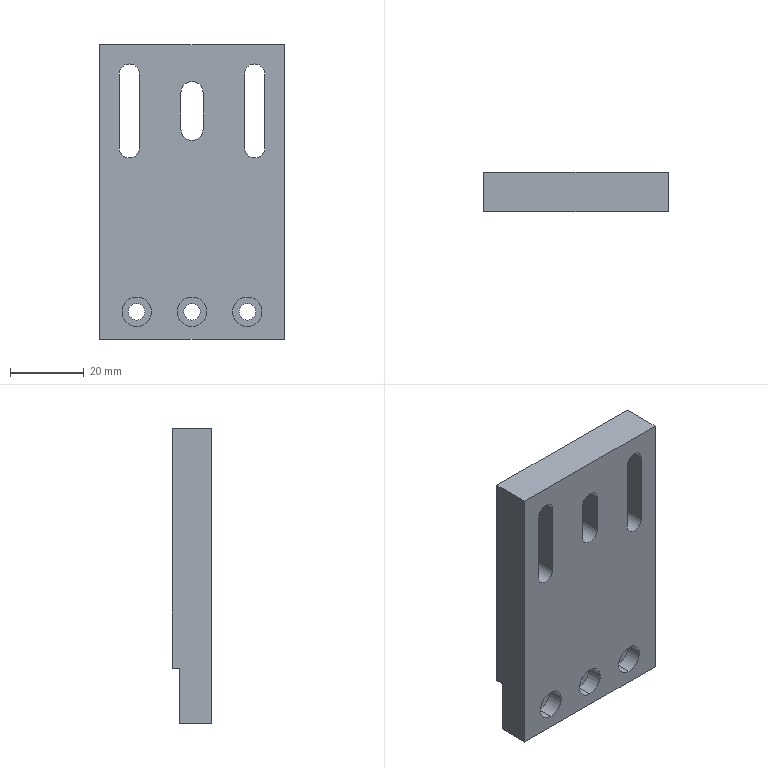Part | STEP file | 05-05 support plate | 1 solid | 50 faces | box 50 x 10.7 x 80 mm | volume 35177 mm3 | cylinder 27 | plane 23 | commonest cylinder face diameters 4.5 x6 5.5 x6 8 x6 10 x6 6 x3
STEP:
#1=CARTESIAN_POINT('',(17.,-5.35,74.75));
#2=VERTEX_POINT('',#1);
#3=CARTESIAN_POINT('',(19.75,-5.35,72.));
#4=VERTEX_POINT('',#3);
#5=CARTESIAN_POINT('',(17.,-5.35,72.));
#6=DIRECTION('',(0.,1.,0.));
#7=DIRECTION('',(0.,0.,1.));
#8=AXIS2_PLACEMENT_3D('',#5,#6,#7);
#9=CIRCLE('',#8,2.75);
#10=EDGE_CURVE('',#2,#4,#9,.T.);
#11=ORIENTED_EDGE('',*,*,#10,.F.);
#12=CARTESIAN_POINT('',(17.,0.35,74.75));
#13=VERTEX_POINT('',#12);
#14=CARTESIAN_POINT('',(17.,-10.65,74.75));
#15=DIRECTION('',(0.,1.,0.));
#16=VECTOR('',#15,1000.);
#17=LINE('',#14,#16);
#18=EDGE_CURVE('',#2,#13,#17,.T.);
#19=ORIENTED_EDGE('',*,*,#18,.T.);
#20=CARTESIAN_POINT('',(19.75,0.35,72.));
#21=VERTEX_POINT('',#20);
#22=CARTESIAN_POINT('',(17.,0.35,72.));
#23=DIRECTION('',(0.,-1.,0.));
#24=DIRECTION('',(0.,0.,-1.));
#25=AXIS2_PLACEMENT_3D('',#22,#23,#24);
#26=CIRCLE('',#25,2.75);
#27=EDGE_CURVE('',#21,#13,#26,.T.);
#28=ORIENTED_EDGE('',*,*,#27,.F.);
#29=CARTESIAN_POINT('',(19.75,-10.65,72.));
#30=DIRECTION('',(0.,1.,0.));
#31=VECTOR('',#30,1000.);
#32=LINE('',#29,#31);
#33=EDGE_CURVE('',#4,#21,#32,.T.);
#34=ORIENTED_EDGE('',*,*,#33,.F.);
#35=EDGE_LOOP('',(#11,#19,#28,#34));
#36=FACE_OUTER_BOUND('',#35,.T.);
#37=CARTESIAN_POINT('',(17.,-10.65,72.));
#38=DIRECTION('',(0.,1.,0.));
#39=DIRECTION('',(0.,0.,1.));
#40=AXIS2_PLACEMENT_3D('',#37,#38,#39);
#41=CYLINDRICAL_SURFACE('',#40,2.75);
#42=ADVANCED_FACE('',(#36),#41,.F.);
#43=CARTESIAN_POINT('',(-17.,-5.35,74.75));
#44=VERTEX_POINT('',#43);
#45=CARTESIAN_POINT('',(-14.25,-5.35,72.));
#46=VERTEX_POINT('',#45);
#47=CARTESIAN_POINT('',(-17.,-5.35,72.));
#48=DIRECTION('',(0.,1.,0.));
#49=DIRECTION('',(0.,0.,1.));
#50=AXIS2_PLACEMENT_3D('',#47,#48,#49);
#51=CIRCLE('',#50,2.75);
#52=EDGE_CURVE('',#44,#46,#51,.T.);
#53=ORIENTED_EDGE('',*,*,#52,.F.);
#54=CARTESIAN_POINT('',(-17.,0.35,74.75));
#55=VERTEX_POINT('',#54);
#56=CARTESIAN_POINT('',(-17.,-10.65,74.75));
#57=DIRECTION('',(0.,1.,0.));
#58=VECTOR('',#57,1000.);
#59=LINE('',#56,#58);
#60=EDGE_CURVE('',#44,#55,#59,.T.);
#61=ORIENTED_EDGE('',*,*,#60,.T.);
#62=CARTESIAN_POINT('',(-14.25,0.35,72.));
#63=VERTEX_POINT('',#62);
#64=CARTESIAN_POINT('',(-17.,0.35,72.));
#65=DIRECTION('',(0.,1.,0.));
#66=DIRECTION('',(0.,0.,1.));
#67=AXIS2_PLACEMENT_3D('',#64,#65,#66);
#68=CIRCLE('',#67,2.75);
#69=EDGE_CURVE('',#55,#63,#68,.T.);
#70=ORIENTED_EDGE('',*,*,#69,.T.);
#71=CARTESIAN_POINT('',(-14.25,-10.65,72.));
#72=DIRECTION('',(0.,1.,0.));
#73=VECTOR('',#72,1000.);
#74=LINE('',#71,#73);
#75=EDGE_CURVE('',#46,#63,#74,.T.);
#76=ORIENTED_EDGE('',*,*,#75,.F.);
#77=EDGE_LOOP('',(#53,#61,#70,#76));
#78=FACE_OUTER_BOUND('',#77,.T.);
#79=CARTESIAN_POINT('',(-17.,-10.65,72.));
#80=DIRECTION('',(0.,1.,0.));
#81=DIRECTION('',(0.,0.,1.));
#82=AXIS2_PLACEMENT_3D('',#79,#80,#81);
#83=CYLINDRICAL_SURFACE('',#82,2.75);
#84=ADVANCED_FACE('',(#78),#83,.F.);
#85=CARTESIAN_POINT('',(0.,-5.35,70.));
#86=VERTEX_POINT('',#85);
#87=CARTESIAN_POINT('',(3.,-5.35,67.));
#88=VERTEX_POINT('',#87);
#89=CARTESIAN_POINT('',(0.,-5.35,67.));
#90=DIRECTION('',(0.,1.,0.));
#91=DIRECTION('',(0.,0.,1.));
#92=AXIS2_PLACEMENT_3D('',#89,#90,#91);
#93=CIRCLE('',#92,3.);
#94=EDGE_CURVE('',#86,#88,#93,.T.);
#95=ORIENTED_EDGE('',*,*,#94,.F.);
#96=CARTESIAN_POINT('',(0.,5.35,70.));
#97=VERTEX_POINT('',#96);
#98=CARTESIAN_POINT('',(0.,-10.65,70.));
#99=DIRECTION('',(0.,1.,0.));
#100=VECTOR('',#99,1000.);
#101=LINE('',#98,#100);
#102=EDGE_CURVE('',#86,#97,#101,.T.);
#103=ORIENTED_EDGE('',*,*,#102,.T.);
#104=CARTESIAN_POINT('',(3.,5.35,67.));
#105=VERTEX_POINT('',#104);
#106=CARTESIAN_POINT('',(0.,5.35,67.));
#107=DIRECTION('',(0.,-1.,0.));
#108=DIRECTION('',(0.,0.,-1.));
#109=AXIS2_PLACEMENT_3D('',#106,#107,#108);
#110=CIRCLE('',#109,3.);
#111=EDGE_CURVE('',#105,#97,#110,.T.);
#112=ORIENTED_EDGE('',*,*,#111,.F.);
#113=CARTESIAN_POINT('',(3.,-10.65,67.));
#114=DIRECTION('',(0.,1.,0.));
#115=VECTOR('',#114,1000.);
#116=LINE('',#113,#115);
#117=EDGE_CURVE('',#88,#105,#116,.T.);
#118=ORIENTED_EDGE('',*,*,#117,.F.);
#119=EDGE_LOOP('',(#95,#103,#112,#118));
#120=FACE_OUTER_BOUND('',#119,.T.);
#121=CARTESIAN_POINT('',(0.,-10.65,67.));
#122=DIRECTION('',(0.,1.,0.));
#123=DIRECTION('',(0.,0.,1.));
#124=AXIS2_PLACEMENT_3D('',#121,#122,#123);
#125=CYLINDRICAL_SURFACE('',#124,3.);
#126=ADVANCED_FACE('',(#120),#125,.F.);
#127=CARTESIAN_POINT('',(17.,0.35,77.));
#128=VERTEX_POINT('',#127);
#129=CARTESIAN_POINT('',(22.,0.35,72.));
#130=VERTEX_POINT('',#129);
#131=CARTESIAN_POINT('',(17.,0.35,72.));
#132=DIRECTION('',(0.,1.,0.));
#133=DIRECTION('',(0.,0.,-1.));
#134=AXIS2_PLACEMENT_3D('',#131,#132,#133);
#135=CIRCLE('',#134,5.);
#136=EDGE_CURVE('',#128,#130,#135,.T.);
#137=ORIENTED_EDGE('',*,*,#136,.F.);
#138=CARTESIAN_POINT('',(17.,5.35,77.));
#139=VERTEX_POINT('',#138);
#140=CARTESIAN_POINT('',(17.,0.35,77.));
#141=DIRECTION('',(0.,1.,0.));
#142=VECTOR('',#141,1000.);
#143=LINE('',#140,#142);
#144=EDGE_CURVE('',#128,#139,#143,.T.);
#145=ORIENTED_EDGE('',*,*,#144,.T.);
#146=CARTESIAN_POINT('',(22.,5.35,72.));
#147=VERTEX_POINT('',#146);
#148=CARTESIAN_POINT('',(17.,5.35,72.));
#149=DIRECTION('',(0.,1.,0.));
#150=DIRECTION('',(0.,0.,-1.));
#151=AXIS2_PLACEMENT_3D('',#148,#149,#150);
#152=CIRCLE('',#151,5.);
#153=EDGE_CURVE('',#139,#147,#152,.T.);
#154=ORIENTED_EDGE('',*,*,#153,.T.);
#155=CARTESIAN_POINT('',(22.,0.35,72.));
#156=DIRECTION('',(0.,1.,0.));
#157=VECTOR('',#156,1000.);
#158=LINE('',#155,#157);
#159=EDGE_CURVE('',#130,#147,#158,.T.);
#160=ORIENTED_EDGE('',*,*,#159,.F.);
#161=EDGE_LOOP('',(#137,#145,#154,#160));
#162=FACE_OUTER_BOUND('',#161,.T.);
#163=CARTESIAN_POINT('',(17.,0.35,72.));
#164=DIRECTION('',(0.,1.,0.));
#165=DIRECTION('',(0.,0.,1.));
#166=AXIS2_PLACEMENT_3D('',#163,#164,#165);
#167=CYLINDRICAL_SURFACE('',#166,5.);
#168=ADVANCED_FACE('',(#162),#167,.F.);
#169=CARTESIAN_POINT('',(-17.,0.35,77.));
#170=VERTEX_POINT('',#169);
#171=CARTESIAN_POINT('',(-12.,0.35,72.));
#172=VERTEX_POINT('',#171);
#173=CARTESIAN_POINT('',(-17.,0.35,72.));
#174=DIRECTION('',(0.,1.,0.));
#175=DIRECTION('',(0.,0.,1.));
#176=AXIS2_PLACEMENT_3D('',#173,#174,#175);
#177=CIRCLE('',#176,5.);
#178=EDGE_CURVE('',#170,#172,#177,.T.);
#179=ORIENTED_EDGE('',*,*,#178,.F.);
#180=CARTESIAN_POINT('',(-17.,5.35,77.));
#181=VERTEX_POINT('',#180);
#182=CARTESIAN_POINT('',(-17.,0.35,77.));
#183=DIRECTION('',(0.,1.,0.));
#184=VECTOR('',#183,1000.);
#185=LINE('',#182,#184);
#186=EDGE_CURVE('',#170,#181,#185,.T.);
#187=ORIENTED_EDGE('',*,*,#186,.T.);
#188=CARTESIAN_POINT('',(-12.,5.35,72.));
#189=VERTEX_POINT('',#188);
#190=CARTESIAN_POINT('',(-17.,5.35,72.));
#191=DIRECTION('',(0.,1.,0.));
#192=DIRECTION('',(0.,0.,1.));
#193=AXIS2_PLACEMENT_3D('',#190,#191,#192);
#194=CIRCLE('',#193,5.);
#195=EDGE_CURVE('',#181,#189,#194,.T.);
#196=ORIENTED_EDGE('',*,*,#195,.T.);
#197=CARTESIAN_POINT('',(-12.,0.35,72.));
#198=DIRECTION('',(0.,1.,0.));
#199=VECTOR('',#198,1000.);
#200=LINE('',#197,#199);
#201=EDGE_CURVE('',#172,#189,#200,.T.);
#202=ORIENTED_EDGE('',*,*,#201,.F.);
#203=EDGE_LOOP('',(#179,#187,#196,#202));
#204=FACE_OUTER_BOUND('',#203,.T.);
#205=CARTESIAN_POINT('',(-17.,0.35,72.));
#206=DIRECTION('',(0.,1.,0.));
#207=DIRECTION('',(0.,0.,1.));
#208=AXIS2_PLACEMENT_3D('',#205,#206,#207);
#209=CYLINDRICAL_SURFACE('',#208,5.);
#210=ADVANCED_FACE('',(#204),#209,.F.);
#211=CARTESIAN_POINT('',(15.,-0.95,11.5));
#212=VERTEX_POINT('',#211);
#213=CARTESIAN_POINT('',(15.,-0.95,3.5));
#214=VERTEX_POINT('',#213);
#215=CARTESIAN_POINT('',(15.,-0.95,7.5));
#216=DIRECTION('',(0.,-1.,0.));
#217=DIRECTION('',(0.,0.,-1.));
#218=AXIS2_PLACEMENT_3D('',#215,#216,#217);
#219=CIRCLE('',#218,4.);
#220=EDGE_CURVE('',#212,#214,#219,.T.);
#221=ORIENTED_EDGE('',*,*,#220,.F.);
#222=CARTESIAN_POINT('',(15.,-5.35,11.5));
#223=VERTEX_POINT('',#222);
#224=CARTESIAN_POINT('',(15.,-5.35,11.5));
#225=DIRECTION('',(0.,-1.,0.));
#226=VECTOR('',#225,1000.);
#227=LINE('',#224,#226);
#228=EDGE_CURVE('',#212,#223,#227,.T.);
#229=ORIENTED_EDGE('',*,*,#228,.T.);
#230=CARTESIAN_POINT('',(15.,-5.35,3.5));
#231=VERTEX_POINT('',#230);
#232=CARTESIAN_POINT('',(15.,-5.35,7.5));
#233=DIRECTION('',(0.,-1.,0.));
#234=DIRECTION('',(0.,0.,-1.));
#235=AXIS2_PLACEMENT_3D('',#232,#233,#234);
#236=CIRCLE('',#235,4.);
#237=EDGE_CURVE('',#223,#231,#236,.T.);
#238=ORIENTED_EDGE('',*,*,#237,.T.);
#239=CARTESIAN_POINT('',(15.,-5.35,3.5));
#240=DIRECTION('',(0.,-1.,0.));
#241=VECTOR('',#240,1000.);
#242=LINE('',#239,#241);
#243=EDGE_CURVE('',#214,#231,#242,.T.);
#244=ORIENTED_EDGE('',*,*,#243,.F.);
#245=EDGE_LOOP('',(#221,#229,#238,#244));
#246=FACE_OUTER_BOUND('',#245,.T.);
#247=CARTESIAN_POINT('',(15.,-5.35,7.5));
#248=DIRECTION('',(0.,-1.,0.));
#249=DIRECTION('',(0.,0.,-1.));
#250=AXIS2_PLACEMENT_3D('',#247,#248,#249);
#251=CYLINDRICAL_SURFACE('',#250,4.);
#252=ADVANCED_FACE('',(#246),#251,.F.);
#253=CARTESIAN_POINT('',(15.,3.35,9.75));
#254=VERTEX_POINT('',#253);
#255=CARTESIAN_POINT('',(15.,3.35,5.25));
#256=VERTEX_POINT('',#255);
#257=CARTESIAN_POINT('',(15.,3.35,7.5));
#258=DIRECTION('',(0.,-1.,0.));
#259=DIRECTION('',(1.,0.,0.));
#260=AXIS2_PLACEMENT_3D('',#257,#258,#259);
#261=CIRCLE('',#260,2.25);
#262=EDGE_CURVE('',#254,#256,#261,.T.);
#263=ORIENTED_EDGE('',*,*,#262,.F.);
#264=CARTESIAN_POINT('',(15.,-0.95,9.75));
#265=VERTEX_POINT('',#264);
#266=CARTESIAN_POINT('',(15.,-5.35,9.75));
#267=DIRECTION('',(0.,-1.,0.));
#268=VECTOR('',#267,1000.);
#269=LINE('',#266,#268);
#270=EDGE_CURVE('',#254,#265,#269,.T.);
#271=ORIENTED_EDGE('',*,*,#270,.T.);
#272=CARTESIAN_POINT('',(15.,-0.95,5.25));
#273=VERTEX_POINT('',#272);
#274=CARTESIAN_POINT('',(15.,-0.95,7.5));
#275=DIRECTION('',(0.,-1.,0.));
#276=DIRECTION('',(0.,0.,-1.));
#277=AXIS2_PLACEMENT_3D('',#274,#275,#276);
#278=CIRCLE('',#277,2.25);
#279=EDGE_CURVE('',#265,#273,#278,.T.);
#280=ORIENTED_EDGE('',*,*,#279,.T.);
#281=CARTESIAN_POINT('',(15.,-5.35,5.25));
#282=DIRECTION('',(0.,-1.,0.));
#283=VECTOR('',#282,1000.);
#284=LINE('',#281,#283);
#285=EDGE_CURVE('',#256,#273,#284,.T.);
#286=ORIENTED_EDGE('',*,*,#285,.F.);
#287=EDGE_LOOP('',(#263,#271,#280,#286));
#288=FACE_OUTER_BOUND('',#287,.T.);
#289=CARTESIAN_POINT('',(15.,-5.35,7.5));
#290=DIRECTION('',(0.,-1.,0.));
#291=DIRECTION('',(0.,0.,-1.));
#292=AXIS2_PLACEMENT_3D('',#289,#290,#291);
#293=CYLINDRICAL_SURFACE('',#292,2.25);
#294=ADVANCED_FACE('',(#288),#293,.F.);
#295=CARTESIAN_POINT('',(0.,-0.95,11.5));
#296=VERTEX_POINT('',#295);
#297=CARTESIAN_POINT('',(0.,-0.95,3.5));
#298=VERTEX_POINT('',#297);
#299=CARTESIAN_POINT('',(0.,-0.95,7.5));
#300=DIRECTION('',(0.,-1.,0.));
#301=DIRECTION('',(0.,0.,-1.));
#302=AXIS2_PLACEMENT_3D('',#299,#300,#301);
#303=CIRCLE('',#302,4.);
#304=EDGE_CURVE('',#296,#298,#303,.T.);
#305=ORIENTED_EDGE('',*,*,#304,.F.);
#306=CARTESIAN_POINT('',(0.,-5.35,11.5));
#307=VERTEX_POINT('',#306);
#308=CARTESIAN_POINT('',(0.,-5.35,11.5));
#309=DIRECTION('',(0.,-1.,0.));
#310=VECTOR('',#309,1000.);
#311=LINE('',#308,#310);
#312=EDGE_CURVE('',#296,#307,#311,.T.);
#313=ORIENTED_EDGE('',*,*,#312,.T.);
#314=CARTESIAN_POINT('',(0.,-5.35,3.5));
#315=VERTEX_POINT('',#314);
#316=CARTESIAN_POINT('',(0.,-5.35,7.5));
#317=DIRECTION('',(0.,-1.,0.));
#318=DIRECTION('',(0.,0.,-1.));
#319=AXIS2_PLACEMENT_3D('',#316,#317,#318);
#320=CIRCLE('',#319,4.);
#321=EDGE_CURVE('',#307,#315,#320,.T.);
#322=ORIENTED_EDGE('',*,*,#321,.T.);
#323=CARTESIAN_POINT('',(0.,-5.35,3.5));
#324=DIRECTION('',(0.,-1.,0.));
#325=VECTOR('',#324,1000.);
#326=LINE('',#323,#325);
#327=EDGE_CURVE('',#298,#315,#326,.T.);
#328=ORIENTED_EDGE('',*,*,#327,.F.);
#329=EDGE_LOOP('',(#305,#313,#322,#328));
#330=FACE_OUTER_BOUND('',#329,.T.);
#331=CARTESIAN_POINT('',(0.,-5.35,7.5));
#332=DIRECTION('',(0.,-1.,0.));
#333=DIRECTION('',(0.,0.,-1.));
#334=AXIS2_PLACEMENT_3D('',#331,#332,#333);
#335=CYLINDRICAL_SURFACE('',#334,4.);
#336=ADVANCED_FACE('',(#330),#335,.F.);
#337=CARTESIAN_POINT('',(0.,3.35,9.75));
#338=VERTEX_POINT('',#337);
#339=CARTESIAN_POINT('',(0.,3.35,5.25));
#340=VERTEX_POINT('',#339);
#341=CARTESIAN_POINT('',(0.,3.35,7.5));
#342=DIRECTION('',(0.,-1.,0.));
#343=DIRECTION('',(1.,0.,0.));
#344=AXIS2_PLACEMENT_3D('',#341,#342,#343);
#345=CIRCLE('',#344,2.25);
#346=EDGE_CURVE('',#338,#340,#345,.T.);
#347=ORIENTED_EDGE('',*,*,#346,.F.);
#348=CARTESIAN_POINT('',(0.,-0.95,9.75));
#349=VERTEX_POINT('',#348);
#350=CARTESIAN_POINT('',(0.,-5.35,9.75));
#351=DIRECTION('',(0.,-1.,0.));
#352=VECTOR('',#351,1000.);
#353=LINE('',#350,#352);
#354=EDGE_CURVE('',#338,#349,#353,.T.);
#355=ORIENTED_EDGE('',*,*,#354,.T.);
#356=CARTESIAN_POINT('',(0.,-0.95,5.25));
#357=VERTEX_POINT('',#356);
#358=CARTESIAN_POINT('',(0.,-0.95,7.5));
#359=DIRECTION('',(0.,-1.,0.));
#360=DIRECTION('',(0.,0.,-1.));
#361=AXIS2_PLACEMENT_3D('',#358,#359,#360);
#362=CIRCLE('',#361,2.25);
#363=EDGE_CURVE('',#349,#357,#362,.T.);
#364=ORIENTED_EDGE('',*,*,#363,.T.);
#365=CARTESIAN_POINT('',(0.,-5.35,5.25));
#366=DIRECTION('',(0.,-1.,0.));
#367=VECTOR('',#366,1000.);
#368=LINE('',#365,#367);
#369=EDGE_CURVE('',#340,#357,#368,.T.);
#370=ORIENTED_EDGE('',*,*,#369,.F.);
#371=EDGE_LOOP('',(#347,#355,#364,#370));
#372=FACE_OUTER_BOUND('',#371,.T.);
#373=CARTESIAN_POINT('',(0.,-5.35,7.5));
#374=DIRECTION('',(0.,-1.,0.));
#375=DIRECTION('',(0.,0.,-1.));
#376=AXIS2_PLACEMENT_3D('',#373,#374,#375);
#377=CYLINDRICAL_SURFACE('',#376,2.25);
#378=ADVANCED_FACE('',(#372),#377,.F.);
#379=CARTESIAN_POINT('',(-15.,-0.95,11.5));
#380=VERTEX_POINT('',#379);
#381=CARTESIAN_POINT('',(-15.,-0.95,3.5));
#382=VERTEX_POINT('',#381);
#383=CARTESIAN_POINT('',(-15.,-0.95,7.5));
#384=DIRECTION('',(0.,-1.,0.));
#385=DIRECTION('',(0.,0.,-1.));
#386=AXIS2_PLACEMENT_3D('',#383,#384,#385);
#387=CIRCLE('',#386,4.);
#388=EDGE_CURVE('',#380,#382,#387,.T.);
#389=ORIENTED_EDGE('',*,*,#388,.F.);
#390=CARTESIAN_POINT('',(-15.,-5.35,11.5));
#391=VERTEX_POINT('',#390);
#392=CARTESIAN_POINT('',(-15.,-5.35,11.5));
#393=DIRECTION('',(0.,-1.,0.));
#394=VECTOR('',#393,1000.);
#395=LINE('',#392,#394);
#396=EDGE_CURVE('',#380,#391,#395,.T.);
#397=ORIENTED_EDGE('',*,*,#396,.T.);
#398=CARTESIAN_POINT('',(-15.,-5.35,3.5));
#399=VERTEX_POINT('',#398);
#400=CARTESIAN_POINT('',(-15.,-5.35,7.5));
#401=DIRECTION('',(0.,-1.,0.));
#402=DIRECTION('',(0.,0.,-1.));
#403=AXIS2_PLACEMENT_3D('',#400,#401,#402);
#404=CIRCLE('',#403,4.);
#405=EDGE_CURVE('',#391,#399,#404,.T.);
#406=ORIENTED_EDGE('',*,*,#405,.T.);
#407=CARTESIAN_POINT('',(-15.,-5.35,3.5));
#408=DIRECTION('',(0.,-1.,0.));
#409=VECTOR('',#408,1000.);
#410=LINE('',#407,#409);
#411=EDGE_CURVE('',#382,#399,#410,.T.);
#412=ORIENTED_EDGE('',*,*,#411,.F.);
#413=EDGE_LOOP('',(#389,#397,#406,#412));
#414=FACE_OUTER_BOUND('',#413,.T.);
#415=CARTESIAN_POINT('',(-15.,-5.35,7.5));
#416=DIRECTION('',(0.,-1.,0.));
#417=DIRECTION('',(0.,0.,-1.));
#418=AXIS2_PLACEMENT_3D('',#415,#416,#417);
#419=CYLINDRICAL_SURFACE('',#418,4.);
#420=ADVANCED_FACE('',(#414),#419,.F.);
#421=CARTESIAN_POINT('',(-15.,3.35,9.75));
#422=VERTEX_POINT('',#421);
#423=CARTESIAN_POINT('',(-15.,3.35,5.25));
#424=VERTEX_POINT('',#423);
#425=CARTESIAN_POINT('',(-15.,3.35,7.5));
#426=DIRECTION('',(0.,-1.,0.));
#427=DIRECTION('',(1.,0.,0.));
#428=AXIS2_PLACEMENT_3D('',#425,#426,#427);
#429=CIRCLE('',#428,2.25);
#430=EDGE_CURVE('',#422,#424,#429,.T.);
#431=ORIENTED_EDGE('',*,*,#430,.F.);
#432=CARTESIAN_POINT('',(-15.,-0.95,9.75));
#433=VERTEX_POINT('',#432);
#434=CARTESIAN_POINT('',(-15.,-5.35,9.75));
#435=DIRECTION('',(0.,-1.,0.));
#436=VECTOR('',#435,1000.);
#437=LINE('',#434,#436);
#438=EDGE_CURVE('',#422,#433,#437,.T.);
#439=ORIENTED_EDGE('',*,*,#438,.T.);
#440=CARTESIAN_POINT('',(-15.,-0.95,5.25));
#441=VERTEX_POINT('',#440);
#442=CARTESIAN_POINT('',(-15.,-0.95,7.5));
#443=DIRECTION('',(0.,-1.,0.));
#444=DIRECTION('',(0.,0.,-1.));
#445=AXIS2_PLACEMENT_3D('',#442,#443,#444);
#446=CIRCLE('',#445,2.25);
#447=EDGE_CURVE('',#433,#441,#446,.T.);
#448=ORIENTED_EDGE('',*,*,#447,.T.);
#449=CARTESIAN_POINT('',(-15.,-5.35,5.25));
#450=DIRECTION('',(0.,-1.,0.));
#451=VECTOR('',#450,1000.);
#452=LINE('',#449,#451);
#453=EDGE_CURVE('',#424,#441,#452,.T.);
#454=ORIENTED_EDGE('',*,*,#453,.F.);
#455=EDGE_LOOP('',(#431,#439,#448,#454));
#456=FACE_OUTER_BOUND('',#455,.T.);
#457=CARTESIAN_POINT('',(-15.,-5.35,7.5));
#458=DIRECTION('',(0.,-1.,0.));
#459=DIRECTION('',(0.,0.,-1.));
#460=AXIS2_PLACEMENT_3D('',#457,#458,#459);
#461=CYLINDRICAL_SURFACE('',#460,2.25);
#462=ADVANCED_FACE('',(#456),#461,.F.);
#463=CARTESIAN_POINT('',(25.,-5.35,0.));
#464=VERTEX_POINT('',#463);
#465=CARTESIAN_POINT('',(25.,3.35,0.));
#466=VERTEX_POINT('',#465);
#467=CARTESIAN_POINT('',(25.,5.35,0.));
#468=DIRECTION('',(0.,1.,0.));
#469=VECTOR('',#468,1000.);
#470=LINE('',#467,#469);
#471=EDGE_CURVE('',#464,#466,#470,.T.);
#472=ORIENTED_EDGE('',*,*,#471,.T.);
#473=CARTESIAN_POINT('',(25.,3.35,15.));
#474=VERTEX_POINT('',#473);
#475=CARTESIAN_POINT('',(25.,3.35,0.));
#476=DIRECTION('',(0.,0.,-1.));
#477=VECTOR('',#476,1000.);
#478=LINE('',#475,#477);
#479=EDGE_CURVE('',#474,#466,#478,.T.);
#480=ORIENTED_EDGE('',*,*,#479,.F.);
#481=CARTESIAN_POINT('',(25.,5.35,15.));
#482=VERTEX_POINT('',#481);
#483=CARTESIAN_POINT('',(25.,5.35,15.));
#484=DIRECTION('',(0.,-1.,0.));
#485=VECTOR('',#484,1000.);
#486=LINE('',#483,#485);
#487=EDGE_CURVE('',#482,#474,#486,.T.);
#488=ORIENTED_EDGE('',*,*,#487,.F.);
#489=CARTESIAN_POINT('',(25.,5.35,80.));
#490=VERTEX_POINT('',#489);
#491=CARTESIAN_POINT('',(25.,5.35,80.));
#492=DIRECTION('',(0.,0.,-1.));
#493=VECTOR('',#492,1000.);
#494=LINE('',#491,#493);
#495=EDGE_CURVE('',#490,#482,#494,.T.);
#496=ORIENTED_EDGE('',*,*,#495,.F.);
#497=CARTESIAN_POINT('',(25.,-5.35,80.));
#498=VERTEX_POINT('',#497);
#499=CARTESIAN_POINT('',(25.,5.35,80.));
#500=DIRECTION('',(0.,1.,0.));
#501=VECTOR('',#500,1000.);
#502=LINE('',#499,#501);
#503=EDGE_CURVE('',#498,#490,#502,.T.);
#504=ORIENTED_EDGE('',*,*,#503,.F.);
#505=CARTESIAN_POINT('',(25.,-5.35,80.));
#506=DIRECTION('',(0.,0.,-1.));
#507=VECTOR('',#506,1000.);
#508=LINE('',#505,#507);
#509=EDGE_CURVE('',#498,#464,#508,.T.);
#510=ORIENTED_EDGE('',*,*,#509,.T.);
#511=EDGE_LOOP('',(#472,#480,#488,#496,#504,#510));
#512=FACE_OUTER_BOUND('',#511,.T.);
#513=CARTESIAN_POINT('',(25.,5.35,80.));
#514=DIRECTION('',(-1.,0.,0.));
#515=DIRECTION('',(0.,-1.,0.));
#516=AXIS2_PLACEMENT_3D('',#513,#514,#515);
#517=PLANE('',#516);
#518=ADVANCED_FACE('',(#512),#517,.F.);
#519=CARTESIAN_POINT('',(-3.,5.35,67.));
#520=VERTEX_POINT('',#519);
#521=CARTESIAN_POINT('',(-3.,5.35,57.));
#522=VERTEX_POINT('',#521);
#523=CARTESIAN_POINT('',(-3.,5.35,80.));
#524=DIRECTION('',(0.,0.,-1.));
#525=VECTOR('',#524,1000.);
#526=LINE('',#523,#525);
#527=EDGE_CURVE('',#520,#522,#526,.T.);
#528=ORIENTED_EDGE('',*,*,#527,.T.);
#529=CARTESIAN_POINT('',(3.,5.35,57.));
#530=VERTEX_POINT('',#529);
#531=CARTESIAN_POINT('',(0.,5.35,57.));
#532=DIRECTION('',(0.,-1.,0.));
#533=DIRECTION('',(0.,0.,-1.));
#534=AXIS2_PLACEMENT_3D('',#531,#532,#533);
#535=CIRCLE('',#534,3.);
#536=EDGE_CURVE('',#522,#530,#535,.T.);
#537=ORIENTED_EDGE('',*,*,#536,.T.);
#538=CARTESIAN_POINT('',(3.,5.35,80.));
#539=DIRECTION('',(0.,0.,1.));
#540=VECTOR('',#539,1000.);
#541=LINE('',#538,#540);
#542=EDGE_CURVE('',#530,#105,#541,.T.);
#543=ORIENTED_EDGE('',*,*,#542,.T.);
#544=ORIENTED_EDGE('',*,*,#111,.T.);
#545=CARTESIAN_POINT('',(0.,5.35,67.));
#546=DIRECTION('',(0.,-1.,0.));
#547=DIRECTION('',(0.,0.,-1.));
#548=AXIS2_PLACEMENT_3D('',#545,#546,#547);
#549=CIRCLE('',#548,3.);
#550=EDGE_CURVE('',#97,#520,#549,.T.);
#551=ORIENTED_EDGE('',*,*,#550,.T.);
#552=EDGE_LOOP('',(#528,#537,#543,#544,#551));
#553=FACE_BOUND('',#552,.T.);
#554=CARTESIAN_POINT('',(12.,5.35,52.));
#555=VERTEX_POINT('',#554);
#556=CARTESIAN_POINT('',(12.,5.35,72.));
#557=VERTEX_POINT('',#556);
#558=CARTESIAN_POINT('',(12.,5.35,52.));
#559=DIRECTION('',(0.,0.,1.));
#560=VECTOR('',#559,1000.);
#561=LINE('',#558,#560);
#562=EDGE_CURVE('',#555,#557,#561,.T.);
#563=ORIENTED_EDGE('',*,*,#562,.F.);
#564=CARTESIAN_POINT('',(22.,5.35,52.));
#565=VERTEX_POINT('',#564);
#566=CARTESIAN_POINT('',(17.,5.35,52.));
#567=DIRECTION('',(0.,1.,0.));
#568=DIRECTION('',(0.,0.,-1.));
#569=AXIS2_PLACEMENT_3D('',#566,#567,#568);
#570=CIRCLE('',#569,5.);
#571=EDGE_CURVE('',#565,#555,#570,.T.);
#572=ORIENTED_EDGE('',*,*,#571,.F.);
#573=CARTESIAN_POINT('',(22.,5.35,52.));
#574=DIRECTION('',(0.,0.,-1.));
#575=VECTOR('',#574,1000.);
#576=LINE('',#573,#575);
#577=EDGE_CURVE('',#147,#565,#576,.T.);
#578=ORIENTED_EDGE('',*,*,#577,.F.);
#579=ORIENTED_EDGE('',*,*,#153,.F.);
#580=CARTESIAN_POINT('',(17.,5.35,72.));
#581=DIRECTION('',(0.,1.,0.));
#582=DIRECTION('',(0.,0.,-1.));
#583=AXIS2_PLACEMENT_3D('',#580,#581,#582);
#584=CIRCLE('',#583,5.);
#585=EDGE_CURVE('',#557,#139,#584,.T.);
#586=ORIENTED_EDGE('',*,*,#585,.F.);
#587=EDGE_LOOP('',(#563,#572,#578,#579,#586));
#588=FACE_BOUND('',#587,.T.);
#589=CARTESIAN_POINT('',(-22.,5.35,52.));
#590=VERTEX_POINT('',#589);
#591=CARTESIAN_POINT('',(-22.,5.35,72.));
#592=VERTEX_POINT('',#591);
#593=CARTESIAN_POINT('',(-22.,5.35,52.));
#594=DIRECTION('',(0.,0.,1.));
#595=VECTOR('',#594,1000.);
#596=LINE('',#593,#595);
#597=EDGE_CURVE('',#590,#592,#596,.T.);
#598=ORIENTED_EDGE('',*,*,#597,.F.);
#599=CARTESIAN_POINT('',(-12.,5.35,52.));
#600=VERTEX_POINT('',#599);
#601=CARTESIAN_POINT('',(-17.,5.35,52.));
#602=DIRECTION('',(0.,1.,0.));
#603=DIRECTION('',(0.,0.,1.));
#604=AXIS2_PLACEMENT_3D('',#601,#602,#603);
#605=CIRCLE('',#604,5.);
#606=EDGE_CURVE('',#600,#590,#605,.T.);
#607=ORIENTED_EDGE('',*,*,#606,.F.);
#608=CARTESIAN_POINT('',(-12.,5.35,52.));
#609=DIRECTION('',(0.,0.,-1.));
#610=VECTOR('',#609,1000.);
#611=LINE('',#608,#610);
#612=EDGE_CURVE('',#189,#600,#611,.T.);
#613=ORIENTED_EDGE('',*,*,#612,.F.);
#614=ORIENTED_EDGE('',*,*,#195,.F.);
#615=CARTESIAN_POINT('',(-17.,5.35,72.));
#616=DIRECTION('',(0.,1.,0.));
#617=DIRECTION('',(0.,0.,1.));
#618=AXIS2_PLACEMENT_3D('',#615,#616,#617);
#619=CIRCLE('',#618,5.);
#620=EDGE_CURVE('',#592,#181,#619,.T.);
#621=ORIENTED_EDGE('',*,*,#620,.F.);
#622=EDGE_LOOP('',(#598,#607,#613,#614,#621));
#623=FACE_BOUND('',#622,.T.);
#624=ORIENTED_EDGE('',*,*,#495,.T.);
#625=CARTESIAN_POINT('',(-25.,5.35,15.));
#626=VERTEX_POINT('',#625);
#627=CARTESIAN_POINT('',(-35.,5.35,15.));
#628=DIRECTION('',(1.,0.,0.));
#629=VECTOR('',#628,1000.);
#630=LINE('',#627,#629);
#631=EDGE_CURVE('',#626,#482,#630,.T.);
#632=ORIENTED_EDGE('',*,*,#631,.F.);
#633=CARTESIAN_POINT('',(-25.,5.35,80.));
#634=VERTEX_POINT('',#633);
#635=CARTESIAN_POINT('',(-25.,5.35,80.));
#636=DIRECTION('',(0.,0.,-1.));
#637=VECTOR('',#636,1000.);
#638=LINE('',#635,#637);
#639=EDGE_CURVE('',#634,#626,#638,.T.);
#640=ORIENTED_EDGE('',*,*,#639,.F.);
#641=CARTESIAN_POINT('',(-25.,5.35,80.));
#642=DIRECTION('',(-1.,0.,0.));
#643=VECTOR('',#642,1000.);
#644=LINE('',#641,#643);
#645=EDGE_CURVE('',#490,#634,#644,.T.);
#646=ORIENTED_EDGE('',*,*,#645,.F.);
#647=EDGE_LOOP('',(#624,#632,#640,#646));
#648=FACE_OUTER_BOUND('',#647,.T.);
#649=CARTESIAN_POINT('',(-25.,5.35,80.));
#650=DIRECTION('',(0.,-1.,0.));
#651=DIRECTION('',(0.,0.,-1.));
#652=AXIS2_PLACEMENT_3D('',#649,#650,#651);
#653=PLANE('',#652);
#654=ADVANCED_FACE('',(#553,#588,#623,#648),#653,.F.);
#655=CARTESIAN_POINT('',(-25.,3.35,15.));
#656=VERTEX_POINT('',#655);
#657=CARTESIAN_POINT('',(-25.,5.35,15.));
#658=DIRECTION('',(0.,-1.,0.));
#659=VECTOR('',#658,1000.);
#660=LINE('',#657,#659);
#661=EDGE_CURVE('',#626,#656,#660,.T.);
#662=ORIENTED_EDGE('',*,*,#661,.T.);
#663=CARTESIAN_POINT('',(-25.,3.35,0.));
#664=VERTEX_POINT('',#663);
#665=CARTESIAN_POINT('',(-25.,3.35,80.));
#666=DIRECTION('',(0.,0.,-1.));
#667=VECTOR('',#666,1000.);
#668=LINE('',#665,#667);
#669=EDGE_CURVE('',#656,#664,#668,.T.);
#670=ORIENTED_EDGE('',*,*,#669,.T.);
#671=CARTESIAN_POINT('',(-25.,-5.35,0.));
#672=VERTEX_POINT('',#671);
#673=CARTESIAN_POINT('',(-25.,5.35,0.));
#674=DIRECTION('',(0.,-1.,0.));
#675=VECTOR('',#674,1000.);
#676=LINE('',#673,#675);
#677=EDGE_CURVE('',#664,#672,#676,.T.);
#678=ORIENTED_EDGE('',*,*,#677,.T.);
#679=CARTESIAN_POINT('',(-25.,-5.35,80.));
#680=VERTEX_POINT('',#679);
#681=CARTESIAN_POINT('',(-25.,-5.35,80.));
#682=DIRECTION('',(0.,0.,-1.));
#683=VECTOR('',#682,1000.);
#684=LINE('',#681,#683);
#685=EDGE_CURVE('',#680,#672,#684,.T.);
#686=ORIENTED_EDGE('',*,*,#685,.F.);
#687=CARTESIAN_POINT('',(-25.,5.35,80.));
#688=DIRECTION('',(0.,-1.,0.));
#689=VECTOR('',#688,1000.);
#690=LINE('',#687,#689);
#691=EDGE_CURVE('',#634,#680,#690,.T.);
#692=ORIENTED_EDGE('',*,*,#691,.F.);
#693=ORIENTED_EDGE('',*,*,#639,.T.);
#694=EDGE_LOOP('',(#662,#670,#678,#686,#692,#693));
#695=FACE_OUTER_BOUND('',#694,.T.);
#696=CARTESIAN_POINT('',(-25.,5.35,80.));
#697=DIRECTION('',(1.,0.,0.));
#698=DIRECTION('',(0.,0.,-1.));
#699=AXIS2_PLACEMENT_3D('',#696,#697,#698);
#700=PLANE('',#699);
#701=ADVANCED_FACE('',(#695),#700,.F.);
#702=CARTESIAN_POINT('',(19.75,-5.35,52.));
#703=VERTEX_POINT('',#702);
#704=CARTESIAN_POINT('',(19.75,-5.35,80.));
#705=DIRECTION('',(0.,0.,-1.));
#706=VECTOR('',#705,1000.);
#707=LINE('',#704,#706);
#708=EDGE_CURVE('',#4,#703,#707,.T.);
#709=ORIENTED_EDGE('',*,*,#708,.T.);
#710=CARTESIAN_POINT('',(14.25,-5.35,52.));
#711=VERTEX_POINT('',#710);
#712=CARTESIAN_POINT('',(17.,-5.35,52.));
#713=DIRECTION('',(0.,1.,0.));
#714=DIRECTION('',(0.,0.,1.));
#715=AXIS2_PLACEMENT_3D('',#712,#713,#714);
#716=CIRCLE('',#715,2.75);
#717=EDGE_CURVE('',#703,#711,#716,.T.);
#718=ORIENTED_EDGE('',*,*,#717,.T.);
#719=CARTESIAN_POINT('',(14.25,-5.35,72.));
#720=VERTEX_POINT('',#719);
#721=CARTESIAN_POINT('',(14.25,-5.35,80.));
#722=DIRECTION('',(0.,0.,1.));
#723=VECTOR('',#722,1000.);
#724=LINE('',#721,#723);
#725=EDGE_CURVE('',#711,#720,#724,.T.);
#726=ORIENTED_EDGE('',*,*,#725,.T.);
#727=CARTESIAN_POINT('',(17.,-5.35,72.));
#728=DIRECTION('',(0.,1.,0.));
#729=DIRECTION('',(0.,0.,1.));
#730=AXIS2_PLACEMENT_3D('',#727,#728,#729);
#731=CIRCLE('',#730,2.75);
#732=EDGE_CURVE('',#720,#2,#731,.T.);
#733=ORIENTED_EDGE('',*,*,#732,.T.);
#734=ORIENTED_EDGE('',*,*,#10,.T.);
#735=EDGE_LOOP('',(#709,#718,#726,#733,#734));
#736=FACE_BOUND('',#735,.T.);
#737=CARTESIAN_POINT('',(-14.25,-5.35,52.));
#738=VERTEX_POINT('',#737);
#739=CARTESIAN_POINT('',(-14.25,-5.35,80.));
#740=DIRECTION('',(0.,0.,-1.));
#741=VECTOR('',#740,1000.);
#742=LINE('',#739,#741);
#743=EDGE_CURVE('',#46,#738,#742,.T.);
#744=ORIENTED_EDGE('',*,*,#743,.T.);
#745=CARTESIAN_POINT('',(-19.75,-5.35,52.));
#746=VERTEX_POINT('',#745);
#747=CARTESIAN_POINT('',(-17.,-5.35,52.));
#748=DIRECTION('',(0.,1.,0.));
#749=DIRECTION('',(0.,0.,1.));
#750=AXIS2_PLACEMENT_3D('',#747,#748,#749);
#751=CIRCLE('',#750,2.75);
#752=EDGE_CURVE('',#738,#746,#751,.T.);
#753=ORIENTED_EDGE('',*,*,#752,.T.);
#754=CARTESIAN_POINT('',(-19.75,-5.35,72.));
#755=VERTEX_POINT('',#754);
#756=CARTESIAN_POINT('',(-19.75,-5.35,80.));
#757=DIRECTION('',(0.,0.,1.));
#758=VECTOR('',#757,1000.);
#759=LINE('',#756,#758);
#760=EDGE_CURVE('',#746,#755,#759,.T.);
#761=ORIENTED_EDGE('',*,*,#760,.T.);
#762=CARTESIAN_POINT('',(-17.,-5.35,72.));
#763=DIRECTION('',(0.,1.,0.));
#764=DIRECTION('',(0.,0.,1.));
#765=AXIS2_PLACEMENT_3D('',#762,#763,#764);
#766=CIRCLE('',#765,2.75);
#767=EDGE_CURVE('',#755,#44,#766,.T.);
#768=ORIENTED_EDGE('',*,*,#767,.T.);
#769=ORIENTED_EDGE('',*,*,#52,.T.);
#770=EDGE_LOOP('',(#744,#753,#761,#768,#769));
#771=FACE_BOUND('',#770,.T.);
#772=CARTESIAN_POINT('',(3.,-5.35,57.));
#773=VERTEX_POINT('',#772);
#774=CARTESIAN_POINT('',(3.,-5.35,80.));
#775=DIRECTION('',(0.,0.,-1.));
#776=VECTOR('',#775,1000.);
#777=LINE('',#774,#776);
#778=EDGE_CURVE('',#88,#773,#777,.T.);
#779=ORIENTED_EDGE('',*,*,#778,.T.);
#780=CARTESIAN_POINT('',(-3.,-5.35,57.));
#781=VERTEX_POINT('',#780);
#782=CARTESIAN_POINT('',(0.,-5.35,57.));
#783=DIRECTION('',(0.,1.,0.));
#784=DIRECTION('',(0.,0.,1.));
#785=AXIS2_PLACEMENT_3D('',#782,#783,#784);
#786=CIRCLE('',#785,3.);
#787=EDGE_CURVE('',#773,#781,#786,.T.);
#788=ORIENTED_EDGE('',*,*,#787,.T.);
#789=CARTESIAN_POINT('',(-3.,-5.35,67.));
#790=VERTEX_POINT('',#789);
#791=CARTESIAN_POINT('',(-3.,-5.35,80.));
#792=DIRECTION('',(0.,0.,1.));
#793=VECTOR('',#792,1000.);
#794=LINE('',#791,#793);
#795=EDGE_CURVE('',#781,#790,#794,.T.);
#796=ORIENTED_EDGE('',*,*,#795,.T.);
#797=CARTESIAN_POINT('',(0.,-5.35,67.));
#798=DIRECTION('',(0.,1.,0.));
#799=DIRECTION('',(0.,0.,1.));
#800=AXIS2_PLACEMENT_3D('',#797,#798,#799);
#801=CIRCLE('',#800,3.);
#802=EDGE_CURVE('',#790,#86,#801,.T.);
#803=ORIENTED_EDGE('',*,*,#802,.T.);
#804=ORIENTED_EDGE('',*,*,#94,.T.);
#805=EDGE_LOOP('',(#779,#788,#796,#803,#804));
#806=FACE_BOUND('',#805,.T.);
#807=CARTESIAN_POINT('',(15.,-5.35,7.5));
#808=DIRECTION('',(0.,-1.,0.));
#809=DIRECTION('',(0.,0.,-1.));
#810=AXIS2_PLACEMENT_3D('',#807,#808,#809);
#811=CIRCLE('',#810,4.);
#812=EDGE_CURVE('',#231,#223,#811,.T.);
#813=ORIENTED_EDGE('',*,*,#812,.F.);
#814=ORIENTED_EDGE('',*,*,#237,.F.);
#815=EDGE_LOOP('',(#813,#814));
#816=FACE_BOUND('',#815,.T.);
#817=CARTESIAN_POINT('',(0.,-5.35,7.5));
#818=DIRECTION('',(0.,-1.,0.));
#819=DIRECTION('',(0.,0.,-1.));
#820=AXIS2_PLACEMENT_3D('',#817,#818,#819);
#821=CIRCLE('',#820,4.);
#822=EDGE_CURVE('',#315,#307,#821,.T.);
#823=ORIENTED_EDGE('',*,*,#822,.F.);
#824=ORIENTED_EDGE('',*,*,#321,.F.);
#825=EDGE_LOOP('',(#823,#824));
#826=FACE_BOUND('',#825,.T.);
#827=CARTESIAN_POINT('',(-15.,-5.35,7.5));
#828=DIRECTION('',(0.,-1.,0.));
#829=DIRECTION('',(0.,0.,-1.));
#830=AXIS2_PLACEMENT_3D('',#827,#828,#829);
#831=CIRCLE('',#830,4.);
#832=EDGE_CURVE('',#399,#391,#831,.T.);
#833=ORIENTED_EDGE('',*,*,#832,.F.);
#834=ORIENTED_EDGE('',*,*,#405,.F.);
#835=EDGE_LOOP('',(#833,#834));
#836=FACE_BOUND('',#835,.T.);
#837=CARTESIAN_POINT('',(-25.,-5.35,0.));
#838=DIRECTION('',(1.,0.,0.));
#839=VECTOR('',#838,1000.);
#840=LINE('',#837,#839);
#841=EDGE_CURVE('',#672,#464,#840,.T.);
#842=ORIENTED_EDGE('',*,*,#841,.T.);
#843=ORIENTED_EDGE('',*,*,#509,.F.);
#844=CARTESIAN_POINT('',(-25.,-5.35,80.));
#845=DIRECTION('',(1.,0.,0.));
#846=VECTOR('',#845,1000.);
#847=LINE('',#844,#846);
#848=EDGE_CURVE('',#680,#498,#847,.T.);
#849=ORIENTED_EDGE('',*,*,#848,.F.);
#850=ORIENTED_EDGE('',*,*,#685,.T.);
#851=EDGE_LOOP('',(#842,#843,#849,#850));
#852=FACE_OUTER_BOUND('',#851,.T.);
#853=CARTESIAN_POINT('',(-25.,-5.35,80.));
#854=DIRECTION('',(0.,1.,0.));
#855=DIRECTION('',(0.,0.,1.));
#856=AXIS2_PLACEMENT_3D('',#853,#854,#855);
#857=PLANE('',#856);
#858=ADVANCED_FACE('',(#736,#771,#806,#816,#826,#836,#852),#857,.F.);
#859=ORIENTED_EDGE('',*,*,#503,.T.);
#860=ORIENTED_EDGE('',*,*,#645,.T.);
#861=ORIENTED_EDGE('',*,*,#691,.T.);
#862=ORIENTED_EDGE('',*,*,#848,.T.);
#863=EDGE_LOOP('',(#859,#860,#861,#862));
#864=FACE_OUTER_BOUND('',#863,.T.);
#865=CARTESIAN_POINT('',(25.,-5.35,80.));
#866=DIRECTION('',(0.,0.,1.));
#867=DIRECTION('',(1.,0.,0.));
#868=AXIS2_PLACEMENT_3D('',#865,#866,#867);
#869=PLANE('',#868);
#870=ADVANCED_FACE('',(#864),#869,.T.);
#871=ORIENTED_EDGE('',*,*,#677,.F.);
#872=CARTESIAN_POINT('',(25.,3.35,0.));
#873=DIRECTION('',(1.,0.,0.));
#874=VECTOR('',#873,1000.);
#875=LINE('',#872,#874);
#876=EDGE_CURVE('',#664,#466,#875,.T.);
#877=ORIENTED_EDGE('',*,*,#876,.T.);
#878=ORIENTED_EDGE('',*,*,#471,.F.);
#879=ORIENTED_EDGE('',*,*,#841,.F.);
#880=EDGE_LOOP('',(#871,#877,#878,#879));
#881=FACE_OUTER_BOUND('',#880,.T.);
#882=CARTESIAN_POINT('',(25.,-5.35,0.));
#883=DIRECTION('',(0.,0.,1.));
#884=DIRECTION('',(1.,0.,0.));
#885=AXIS2_PLACEMENT_3D('',#882,#883,#884);
#886=PLANE('',#885);
#887=ADVANCED_FACE('',(#881),#886,.F.);
#888=ORIENTED_EDGE('',*,*,#631,.T.);
#889=ORIENTED_EDGE('',*,*,#487,.T.);
#890=CARTESIAN_POINT('',(-35.,3.35,15.));
#891=DIRECTION('',(1.,0.,0.));
#892=VECTOR('',#891,1000.);
#893=LINE('',#890,#892);
#894=EDGE_CURVE('',#656,#474,#893,.T.);
#895=ORIENTED_EDGE('',*,*,#894,.F.);
#896=ORIENTED_EDGE('',*,*,#661,.F.);
#897=EDGE_LOOP('',(#888,#889,#895,#896));
#898=FACE_OUTER_BOUND('',#897,.T.);
#899=CARTESIAN_POINT('',(-35.,5.35,15.));
#900=DIRECTION('',(0.,0.,1.));
#901=DIRECTION('',(1.,0.,0.));
#902=AXIS2_PLACEMENT_3D('',#899,#900,#901);
#903=PLANE('',#902);
#904=ADVANCED_FACE('',(#898),#903,.F.);
#905=CARTESIAN_POINT('',(15.,3.35,7.5));
#906=DIRECTION('',(0.,-1.,0.));
#907=DIRECTION('',(1.,0.,0.));
#908=AXIS2_PLACEMENT_3D('',#905,#906,#907);
#909=CIRCLE('',#908,2.25);
#910=EDGE_CURVE('',#256,#254,#909,.T.);
#911=ORIENTED_EDGE('',*,*,#910,.T.);
#912=ORIENTED_EDGE('',*,*,#262,.T.);
#913=EDGE_LOOP('',(#911,#912));
#914=FACE_BOUND('',#913,.T.);
#915=CARTESIAN_POINT('',(0.,3.35,7.5));
#916=DIRECTION('',(0.,-1.,0.));
#917=DIRECTION('',(1.,0.,0.));
#918=AXIS2_PLACEMENT_3D('',#915,#916,#917);
#919=CIRCLE('',#918,2.25);
#920=EDGE_CURVE('',#340,#338,#919,.T.);
#921=ORIENTED_EDGE('',*,*,#920,.T.);
#922=ORIENTED_EDGE('',*,*,#346,.T.);
#923=EDGE_LOOP('',(#921,#922));
#924=FACE_BOUND('',#923,.T.);
#925=CARTESIAN_POINT('',(-15.,3.35,7.5));
#926=DIRECTION('',(0.,-1.,0.));
#927=DIRECTION('',(1.,0.,0.));
#928=AXIS2_PLACEMENT_3D('',#925,#926,#927);
#929=CIRCLE('',#928,2.25);
#930=EDGE_CURVE('',#424,#422,#929,.T.);
#931=ORIENTED_EDGE('',*,*,#930,.T.);
#932=ORIENTED_EDGE('',*,*,#430,.T.);
#933=EDGE_LOOP('',(#931,#932));
#934=FACE_BOUND('',#933,.T.);
#935=ORIENTED_EDGE('',*,*,#894,.T.);
#936=ORIENTED_EDGE('',*,*,#479,.T.);
#937=ORIENTED_EDGE('',*,*,#876,.F.);
#938=ORIENTED_EDGE('',*,*,#669,.F.);
#939=EDGE_LOOP('',(#935,#936,#937,#938));
#940=FACE_OUTER_BOUND('',#939,.T.);
#941=CARTESIAN_POINT('',(-35.,3.35,0.));
#942=DIRECTION('',(0.,-1.,0.));
#943=DIRECTION('',(1.,0.,0.));
#944=AXIS2_PLACEMENT_3D('',#941,#942,#943);
#945=PLANE('',#944);
#946=ADVANCED_FACE('',(#914,#924,#934,#940),#945,.F.);
#947=ORIENTED_EDGE('',*,*,#438,.F.);
#948=ORIENTED_EDGE('',*,*,#930,.F.);
#949=ORIENTED_EDGE('',*,*,#453,.T.);
#950=CARTESIAN_POINT('',(-15.,-0.95,7.5));
#951=DIRECTION('',(0.,-1.,0.));
#952=DIRECTION('',(0.,0.,-1.));
#953=AXIS2_PLACEMENT_3D('',#950,#951,#952);
#954=CIRCLE('',#953,2.25);
#955=EDGE_CURVE('',#441,#433,#954,.T.);
#956=ORIENTED_EDGE('',*,*,#955,.T.);
#957=EDGE_LOOP('',(#947,#948,#949,#956));
#958=FACE_OUTER_BOUND('',#957,.T.);
#959=CARTESIAN_POINT('',(-15.,-5.35,7.5));
#960=DIRECTION('',(0.,-1.,0.));
#961=DIRECTION('',(0.,0.,-1.));
#962=AXIS2_PLACEMENT_3D('',#959,#960,#961);
#963=CYLINDRICAL_SURFACE('',#962,2.25);
#964=ADVANCED_FACE('',(#958),#963,.F.);
#965=ORIENTED_EDGE('',*,*,#955,.F.);
#966=ORIENTED_EDGE('',*,*,#447,.F.);
#967=EDGE_LOOP('',(#965,#966));
#968=FACE_BOUND('',#967,.T.);
#969=CARTESIAN_POINT('',(-15.,-0.95,7.5));
#970=DIRECTION('',(0.,-1.,0.));
#971=DIRECTION('',(0.,0.,-1.));
#972=AXIS2_PLACEMENT_3D('',#969,#970,#971);
#973=CIRCLE('',#972,4.);
#974=EDGE_CURVE('',#382,#380,#973,.T.);
#975=ORIENTED_EDGE('',*,*,#974,.T.);
#976=ORIENTED_EDGE('',*,*,#388,.T.);
#977=EDGE_LOOP('',(#975,#976));
#978=FACE_OUTER_BOUND('',#977,.T.);
#979=CARTESIAN_POINT('',(-12.75,-0.95,7.5));
#980=DIRECTION('',(0.,1.,0.));
#981=DIRECTION('',(0.,0.,1.));
#982=AXIS2_PLACEMENT_3D('',#979,#980,#981);
#983=PLANE('',#982);
#984=ADVANCED_FACE('',(#968,#978),#983,.F.);
#985=ORIENTED_EDGE('',*,*,#396,.F.);
#986=ORIENTED_EDGE('',*,*,#974,.F.);
#987=ORIENTED_EDGE('',*,*,#411,.T.);
#988=ORIENTED_EDGE('',*,*,#832,.T.);
#989=EDGE_LOOP('',(#985,#986,#987,#988));
#990=FACE_OUTER_BOUND('',#989,.T.);
#991=CARTESIAN_POINT('',(-15.,-5.35,7.5));
#992=DIRECTION('',(0.,-1.,0.));
#993=DIRECTION('',(0.,0.,-1.));
#994=AXIS2_PLACEMENT_3D('',#991,#992,#993);
#995=CYLINDRICAL_SURFACE('',#994,4.);
#996=ADVANCED_FACE('',(#990),#995,.F.);
#997=ORIENTED_EDGE('',*,*,#354,.F.);
#998=ORIENTED_EDGE('',*,*,#920,.F.);
#999=ORIENTED_EDGE('',*,*,#369,.T.);
#1000=CARTESIAN_POINT('',(0.,-0.95,7.5));
#1001=DIRECTION('',(0.,-1.,0.));
#1002=DIRECTION('',(0.,0.,-1.));
#1003=AXIS2_PLACEMENT_3D('',#1000,#1001,#1002);
#1004=CIRCLE('',#1003,2.25);
#1005=EDGE_CURVE('',#357,#349,#1004,.T.);
#1006=ORIENTED_EDGE('',*,*,#1005,.T.);
#1007=EDGE_LOOP('',(#997,#998,#999,#1006));
#1008=FACE_OUTER_BOUND('',#1007,.T.);
#1009=CARTESIAN_POINT('',(0.,-5.35,7.5));
#1010=DIRECTION('',(0.,-1.,0.));
#1011=DIRECTION('',(0.,0.,-1.));
#1012=AXIS2_PLACEMENT_3D('',#1009,#1010,#1011);
#1013=CYLINDRICAL_SURFACE('',#1012,2.25);
#1014=ADVANCED_FACE('',(#1008),#1013,.F.);
#1015=ORIENTED_EDGE('',*,*,#1005,.F.);
#1016=ORIENTED_EDGE('',*,*,#363,.F.);
#1017=EDGE_LOOP('',(#1015,#1016));
#1018=FACE_BOUND('',#1017,.T.);
#1019=CARTESIAN_POINT('',(0.,-0.95,7.5));
#1020=DIRECTION('',(0.,-1.,0.));
#1021=DIRECTION('',(0.,0.,-1.));
#1022=AXIS2_PLACEMENT_3D('',#1019,#1020,#1021);
#1023=CIRCLE('',#1022,4.);
#1024=EDGE_CURVE('',#298,#296,#1023,.T.);
#1025=ORIENTED_EDGE('',*,*,#1024,.T.);
#1026=ORIENTED_EDGE('',*,*,#304,.T.);
#1027=EDGE_LOOP('',(#1025,#1026));
#1028=FACE_OUTER_BOUND('',#1027,.T.);
#1029=CARTESIAN_POINT('',(2.25,-0.95,7.5));
#1030=DIRECTION('',(0.,1.,0.));
#1031=DIRECTION('',(0.,0.,1.));
#1032=AXIS2_PLACEMENT_3D('',#1029,#1030,#1031);
#1033=PLANE('',#1032);
#1034=ADVANCED_FACE('',(#1018,#1028),#1033,.F.);
#1035=ORIENTED_EDGE('',*,*,#312,.F.);
#1036=ORIENTED_EDGE('',*,*,#1024,.F.);
#1037=ORIENTED_EDGE('',*,*,#327,.T.);
#1038=ORIENTED_EDGE('',*,*,#822,.T.);
#1039=EDGE_LOOP('',(#1035,#1036,#1037,#1038));
#1040=FACE_OUTER_BOUND('',#1039,.T.);
#1041=CARTESIAN_POINT('',(0.,-5.35,7.5));
#1042=DIRECTION('',(0.,-1.,0.));
#1043=DIRECTION('',(0.,0.,-1.));
#1044=AXIS2_PLACEMENT_3D('',#1041,#1042,#1043);
#1045=CYLINDRICAL_SURFACE('',#1044,4.);
#1046=ADVANCED_FACE('',(#1040),#1045,.F.);
#1047=ORIENTED_EDGE('',*,*,#270,.F.);
#1048=ORIENTED_EDGE('',*,*,#910,.F.);
#1049=ORIENTED_EDGE('',*,*,#285,.T.);
#1050=CARTESIAN_POINT('',(15.,-0.95,7.5));
#1051=DIRECTION('',(0.,-1.,0.));
#1052=DIRECTION('',(0.,0.,-1.));
#1053=AXIS2_PLACEMENT_3D('',#1050,#1051,#1052);
#1054=CIRCLE('',#1053,2.25);
#1055=EDGE_CURVE('',#273,#265,#1054,.T.);
#1056=ORIENTED_EDGE('',*,*,#1055,.T.);
#1057=EDGE_LOOP('',(#1047,#1048,#1049,#1056));
#1058=FACE_OUTER_BOUND('',#1057,.T.);
#1059=CARTESIAN_POINT('',(15.,-5.35,7.5));
#1060=DIRECTION('',(0.,-1.,0.));
#1061=DIRECTION('',(0.,0.,-1.));
#1062=AXIS2_PLACEMENT_3D('',#1059,#1060,#1061);
#1063=CYLINDRICAL_SURFACE('',#1062,2.25);
#1064=ADVANCED_FACE('',(#1058),#1063,.F.);
#1065=ORIENTED_EDGE('',*,*,#1055,.F.);
#1066=ORIENTED_EDGE('',*,*,#279,.F.);
#1067=EDGE_LOOP('',(#1065,#1066));
#1068=FACE_BOUND('',#1067,.T.);
#1069=CARTESIAN_POINT('',(15.,-0.95,7.5));
#1070=DIRECTION('',(0.,-1.,0.));
#1071=DIRECTION('',(0.,0.,-1.));
#1072=AXIS2_PLACEMENT_3D('',#1069,#1070,#1071);
#1073=CIRCLE('',#1072,4.);
#1074=EDGE_CURVE('',#214,#212,#1073,.T.);
#1075=ORIENTED_EDGE('',*,*,#1074,.T.);
#1076=ORIENTED_EDGE('',*,*,#220,.T.);
#1077=EDGE_LOOP('',(#1075,#1076));
#1078=FACE_OUTER_BOUND('',#1077,.T.);
#1079=CARTESIAN_POINT('',(17.25,-0.95,7.5));
#1080=DIRECTION('',(0.,1.,0.));
#1081=DIRECTION('',(0.,0.,1.));
#1082=AXIS2_PLACEMENT_3D('',#1079,#1080,#1081);
#1083=PLANE('',#1082);
#1084=ADVANCED_FACE('',(#1068,#1078),#1083,.F.);
#1085=ORIENTED_EDGE('',*,*,#228,.F.);
#1086=ORIENTED_EDGE('',*,*,#1074,.F.);
#1087=ORIENTED_EDGE('',*,*,#243,.T.);
#1088=ORIENTED_EDGE('',*,*,#812,.T.);
#1089=EDGE_LOOP('',(#1085,#1086,#1087,#1088));
#1090=FACE_OUTER_BOUND('',#1089,.T.);
#1091=CARTESIAN_POINT('',(15.,-5.35,7.5));
#1092=DIRECTION('',(0.,-1.,0.));
#1093=DIRECTION('',(0.,0.,-1.));
#1094=AXIS2_PLACEMENT_3D('',#1091,#1092,#1093);
#1095=CYLINDRICAL_SURFACE('',#1094,4.);
#1096=ADVANCED_FACE('',(#1090),#1095,.F.);
#1097=ORIENTED_EDGE('',*,*,#606,.T.);
#1098=CARTESIAN_POINT('',(-22.,0.35,52.));
#1099=VERTEX_POINT('',#1098);
#1100=CARTESIAN_POINT('',(-22.,0.35,52.));
#1101=DIRECTION('',(0.,1.,0.));
#1102=VECTOR('',#1101,1000.);
#1103=LINE('',#1100,#1102);
#1104=EDGE_CURVE('',#1099,#590,#1103,.T.);
#1105=ORIENTED_EDGE('',*,*,#1104,.F.);
#1106=CARTESIAN_POINT('',(-12.,0.35,52.));
#1107=VERTEX_POINT('',#1106);
#1108=CARTESIAN_POINT('',(-17.,0.35,52.));
#1109=DIRECTION('',(0.,1.,0.));
#1110=DIRECTION('',(0.,0.,1.));
#1111=AXIS2_PLACEMENT_3D('',#1108,#1109,#1110);
#1112=CIRCLE('',#1111,5.);
#1113=EDGE_CURVE('',#1107,#1099,#1112,.T.);
#1114=ORIENTED_EDGE('',*,*,#1113,.F.);
#1115=CARTESIAN_POINT('',(-12.,0.35,52.));
#1116=DIRECTION('',(0.,1.,0.));
#1117=VECTOR('',#1116,1000.);
#1118=LINE('',#1115,#1117);
#1119=EDGE_CURVE('',#1107,#600,#1118,.T.);
#1120=ORIENTED_EDGE('',*,*,#1119,.T.);
#1121=EDGE_LOOP('',(#1097,#1105,#1114,#1120));
#1122=FACE_OUTER_BOUND('',#1121,.T.);
#1123=CARTESIAN_POINT('',(-17.,0.35,52.));
#1124=DIRECTION('',(0.,1.,0.));
#1125=DIRECTION('',(0.,0.,1.));
#1126=AXIS2_PLACEMENT_3D('',#1123,#1124,#1125);
#1127=CYLINDRICAL_SURFACE('',#1126,5.);
#1128=ADVANCED_FACE('',(#1122),#1127,.F.);
#1129=ORIENTED_EDGE('',*,*,#612,.T.);
#1130=ORIENTED_EDGE('',*,*,#1119,.F.);
#1131=CARTESIAN_POINT('',(-12.,0.35,52.));
#1132=DIRECTION('',(0.,0.,-1.));
#1133=VECTOR('',#1132,1000.);
#1134=LINE('',#1131,#1133);
#1135=EDGE_CURVE('',#172,#1107,#1134,.T.);
#1136=ORIENTED_EDGE('',*,*,#1135,.F.);
#1137=ORIENTED_EDGE('',*,*,#201,.T.);
#1138=EDGE_LOOP('',(#1129,#1130,#1136,#1137));
#1139=FACE_OUTER_BOUND('',#1138,.T.);
#1140=CARTESIAN_POINT('',(-12.,0.35,52.));
#1141=DIRECTION('',(1.,0.,0.));
#1142=DIRECTION('',(0.,0.,-1.));
#1143=AXIS2_PLACEMENT_3D('',#1140,#1141,#1142);
#1144=PLANE('',#1143);
#1145=ADVANCED_FACE('',(#1139),#1144,.F.);
#1146=ORIENTED_EDGE('',*,*,#186,.F.);
#1147=CARTESIAN_POINT('',(-22.,0.35,72.));
#1148=VERTEX_POINT('',#1147);
#1149=CARTESIAN_POINT('',(-17.,0.35,72.));
#1150=DIRECTION('',(0.,1.,0.));
#1151=DIRECTION('',(0.,0.,1.));
#1152=AXIS2_PLACEMENT_3D('',#1149,#1150,#1151);
#1153=CIRCLE('',#1152,5.);
#1154=EDGE_CURVE('',#1148,#170,#1153,.T.);
#1155=ORIENTED_EDGE('',*,*,#1154,.F.);
#1156=CARTESIAN_POINT('',(-22.,0.35,72.));
#1157=DIRECTION('',(0.,1.,0.));
#1158=VECTOR('',#1157,1000.);
#1159=LINE('',#1156,#1158);
#1160=EDGE_CURVE('',#1148,#592,#1159,.T.);
#1161=ORIENTED_EDGE('',*,*,#1160,.T.);
#1162=ORIENTED_EDGE('',*,*,#620,.T.);
#1163=EDGE_LOOP('',(#1146,#1155,#1161,#1162));
#1164=FACE_OUTER_BOUND('',#1163,.T.);
#1165=CARTESIAN_POINT('',(-17.,0.35,72.));
#1166=DIRECTION('',(0.,1.,0.));
#1167=DIRECTION('',(0.,0.,1.));
#1168=AXIS2_PLACEMENT_3D('',#1165,#1166,#1167);
#1169=CYLINDRICAL_SURFACE('',#1168,5.);
#1170=ADVANCED_FACE('',(#1164),#1169,.F.);
#1171=ORIENTED_EDGE('',*,*,#597,.T.);
#1172=ORIENTED_EDGE('',*,*,#1160,.F.);
#1173=CARTESIAN_POINT('',(-22.,0.35,52.));
#1174=DIRECTION('',(0.,0.,1.));
#1175=VECTOR('',#1174,1000.);
#1176=LINE('',#1173,#1175);
#1177=EDGE_CURVE('',#1099,#1148,#1176,.T.);
#1178=ORIENTED_EDGE('',*,*,#1177,.F.);
#1179=ORIENTED_EDGE('',*,*,#1104,.T.);
#1180=EDGE_LOOP('',(#1171,#1172,#1178,#1179));
#1181=FACE_OUTER_BOUND('',#1180,.T.);
#1182=CARTESIAN_POINT('',(-22.,0.35,52.));
#1183=DIRECTION('',(-1.,0.,0.));
#1184=DIRECTION('',(0.,0.,1.));
#1185=AXIS2_PLACEMENT_3D('',#1182,#1183,#1184);
#1186=PLANE('',#1185);
#1187=ADVANCED_FACE('',(#1181),#1186,.F.);
#1188=CARTESIAN_POINT('',(-14.25,0.35,52.));
#1189=VERTEX_POINT('',#1188);
#1190=CARTESIAN_POINT('',(-19.75,0.35,52.));
#1191=VERTEX_POINT('',#1190);
#1192=CARTESIAN_POINT('',(-17.,0.35,52.));
#1193=DIRECTION('',(0.,1.,0.));
#1194=DIRECTION('',(0.,0.,1.));
#1195=AXIS2_PLACEMENT_3D('',#1192,#1193,#1194);
#1196=CIRCLE('',#1195,2.75);
#1197=EDGE_CURVE('',#1189,#1191,#1196,.T.);
#1198=ORIENTED_EDGE('',*,*,#1197,.F.);
#1199=CARTESIAN_POINT('',(-14.25,0.35,52.));
#1200=DIRECTION('',(0.,0.,-1.));
#1201=VECTOR('',#1200,1000.);
#1202=LINE('',#1199,#1201);
#1203=EDGE_CURVE('',#63,#1189,#1202,.T.);
#1204=ORIENTED_EDGE('',*,*,#1203,.F.);
#1205=ORIENTED_EDGE('',*,*,#69,.F.);
#1206=CARTESIAN_POINT('',(-19.75,0.35,72.));
#1207=VERTEX_POINT('',#1206);
#1208=CARTESIAN_POINT('',(-17.,0.35,72.));
#1209=DIRECTION('',(0.,1.,0.));
#1210=DIRECTION('',(0.,0.,1.));
#1211=AXIS2_PLACEMENT_3D('',#1208,#1209,#1210);
#1212=CIRCLE('',#1211,2.75);
#1213=EDGE_CURVE('',#1207,#55,#1212,.T.);
#1214=ORIENTED_EDGE('',*,*,#1213,.F.);
#1215=CARTESIAN_POINT('',(-19.75,0.35,52.));
#1216=DIRECTION('',(0.,0.,1.));
#1217=VECTOR('',#1216,1000.);
#1218=LINE('',#1215,#1217);
#1219=EDGE_CURVE('',#1191,#1207,#1218,.T.);
#1220=ORIENTED_EDGE('',*,*,#1219,.F.);
#1221=EDGE_LOOP('',(#1198,#1204,#1205,#1214,#1220));
#1222=FACE_BOUND('',#1221,.T.);
#1223=ORIENTED_EDGE('',*,*,#1113,.T.);
#1224=ORIENTED_EDGE('',*,*,#1177,.T.);
#1225=ORIENTED_EDGE('',*,*,#1154,.T.);
#1226=ORIENTED_EDGE('',*,*,#178,.T.);
#1227=ORIENTED_EDGE('',*,*,#1135,.T.);
#1228=EDGE_LOOP('',(#1223,#1224,#1225,#1226,#1227));
#1229=FACE_OUTER_BOUND('',#1228,.T.);
#1230=CARTESIAN_POINT('',(-17.,0.35,52.));
#1231=DIRECTION('',(0.,1.,0.));
#1232=DIRECTION('',(0.,0.,1.));
#1233=AXIS2_PLACEMENT_3D('',#1230,#1231,#1232);
#1234=PLANE('',#1233);
#1235=ADVANCED_FACE('',(#1222,#1229),#1234,.T.);
#1236=ORIENTED_EDGE('',*,*,#571,.T.);
#1237=CARTESIAN_POINT('',(12.,0.35,52.));
#1238=VERTEX_POINT('',#1237);
#1239=CARTESIAN_POINT('',(12.,0.35,52.));
#1240=DIRECTION('',(0.,1.,0.));
#1241=VECTOR('',#1240,1000.);
#1242=LINE('',#1239,#1241);
#1243=EDGE_CURVE('',#1238,#555,#1242,.T.);
#1244=ORIENTED_EDGE('',*,*,#1243,.F.);
#1245=CARTESIAN_POINT('',(22.,0.35,52.));
#1246=VERTEX_POINT('',#1245);
#1247=CARTESIAN_POINT('',(17.,0.35,52.));
#1248=DIRECTION('',(0.,1.,0.));
#1249=DIRECTION('',(0.,0.,-1.));
#1250=AXIS2_PLACEMENT_3D('',#1247,#1248,#1249);
#1251=CIRCLE('',#1250,5.);
#1252=EDGE_CURVE('',#1246,#1238,#1251,.T.);
#1253=ORIENTED_EDGE('',*,*,#1252,.F.);
#1254=CARTESIAN_POINT('',(22.,0.35,52.));
#1255=DIRECTION('',(0.,1.,0.));
#1256=VECTOR('',#1255,1000.);
#1257=LINE('',#1254,#1256);
#1258=EDGE_CURVE('',#1246,#565,#1257,.T.);
#1259=ORIENTED_EDGE('',*,*,#1258,.T.);
#1260=EDGE_LOOP('',(#1236,#1244,#1253,#1259));
#1261=FACE_OUTER_BOUND('',#1260,.T.);
#1262=CARTESIAN_POINT('',(17.,0.35,52.));
#1263=DIRECTION('',(0.,1.,0.));
#1264=DIRECTION('',(0.,0.,1.));
#1265=AXIS2_PLACEMENT_3D('',#1262,#1263,#1264);
#1266=CYLINDRICAL_SURFACE('',#1265,5.);
#1267=ADVANCED_FACE('',(#1261),#1266,.F.);
#1268=ORIENTED_EDGE('',*,*,#577,.T.);
#1269=ORIENTED_EDGE('',*,*,#1258,.F.);
#1270=CARTESIAN_POINT('',(22.,0.35,52.));
#1271=DIRECTION('',(0.,0.,-1.));
#1272=VECTOR('',#1271,1000.);
#1273=LINE('',#1270,#1272);
#1274=EDGE_CURVE('',#130,#1246,#1273,.T.);
#1275=ORIENTED_EDGE('',*,*,#1274,.F.);
#1276=ORIENTED_EDGE('',*,*,#159,.T.);
#1277=EDGE_LOOP('',(#1268,#1269,#1275,#1276));
#1278=FACE_OUTER_BOUND('',#1277,.T.);
#1279=CARTESIAN_POINT('',(22.,0.35,52.));
#1280=DIRECTION('',(1.,0.,0.));
#1281=DIRECTION('',(0.,0.,-1.));
#1282=AXIS2_PLACEMENT_3D('',#1279,#1280,#1281);
#1283=PLANE('',#1282);
#1284=ADVANCED_FACE('',(#1278),#1283,.F.);
#1285=ORIENTED_EDGE('',*,*,#144,.F.);
#1286=CARTESIAN_POINT('',(12.,0.35,72.));
#1287=VERTEX_POINT('',#1286);
#1288=CARTESIAN_POINT('',(17.,0.35,72.));
#1289=DIRECTION('',(0.,1.,0.));
#1290=DIRECTION('',(0.,0.,-1.));
#1291=AXIS2_PLACEMENT_3D('',#1288,#1289,#1290);
#1292=CIRCLE('',#1291,5.);
#1293=EDGE_CURVE('',#1287,#128,#1292,.T.);
#1294=ORIENTED_EDGE('',*,*,#1293,.F.);
#1295=CARTESIAN_POINT('',(12.,0.35,72.));
#1296=DIRECTION('',(0.,1.,0.));
#1297=VECTOR('',#1296,1000.);
#1298=LINE('',#1295,#1297);
#1299=EDGE_CURVE('',#1287,#557,#1298,.T.);
#1300=ORIENTED_EDGE('',*,*,#1299,.T.);
#1301=ORIENTED_EDGE('',*,*,#585,.T.);
#1302=EDGE_LOOP('',(#1285,#1294,#1300,#1301));
#1303=FACE_OUTER_BOUND('',#1302,.T.);
#1304=CARTESIAN_POINT('',(17.,0.35,72.));
#1305=DIRECTION('',(0.,1.,0.));
#1306=DIRECTION('',(0.,0.,1.));
#1307=AXIS2_PLACEMENT_3D('',#1304,#1305,#1306);
#1308=CYLINDRICAL_SURFACE('',#1307,5.);
#1309=ADVANCED_FACE('',(#1303),#1308,.F.);
#1310=ORIENTED_EDGE('',*,*,#562,.T.);
#1311=ORIENTED_EDGE('',*,*,#1299,.F.);
#1312=CARTESIAN_POINT('',(12.,0.35,52.));
#1313=DIRECTION('',(0.,0.,1.));
#1314=VECTOR('',#1313,1000.);
#1315=LINE('',#1312,#1314);
#1316=EDGE_CURVE('',#1238,#1287,#1315,.T.);
#1317=ORIENTED_EDGE('',*,*,#1316,.F.);
#1318=ORIENTED_EDGE('',*,*,#1243,.T.);
#1319=EDGE_LOOP('',(#1310,#1311,#1317,#1318));
#1320=FACE_OUTER_BOUND('',#1319,.T.);
#1321=CARTESIAN_POINT('',(12.,0.35,52.));
#1322=DIRECTION('',(-1.,0.,0.));
#1323=DIRECTION('',(0.,0.,1.));
#1324=AXIS2_PLACEMENT_3D('',#1321,#1322,#1323);
#1325=PLANE('',#1324);
#1326=ADVANCED_FACE('',(#1320),#1325,.F.);
#1327=CARTESIAN_POINT('',(14.25,0.35,72.));
#1328=VERTEX_POINT('',#1327);
#1329=CARTESIAN_POINT('',(14.25,0.35,52.));
#1330=VERTEX_POINT('',#1329);
#1331=CARTESIAN_POINT('',(14.25,0.35,52.));
#1332=DIRECTION('',(0.,0.,-1.));
#1333=VECTOR('',#1332,1000.);
#1334=LINE('',#1331,#1333);
#1335=EDGE_CURVE('',#1328,#1330,#1334,.T.);
#1336=ORIENTED_EDGE('',*,*,#1335,.T.);
#1337=CARTESIAN_POINT('',(19.75,0.35,52.));
#1338=VERTEX_POINT('',#1337);
#1339=CARTESIAN_POINT('',(17.,0.35,52.));
#1340=DIRECTION('',(0.,-1.,0.));
#1341=DIRECTION('',(0.,0.,-1.));
#1342=AXIS2_PLACEMENT_3D('',#1339,#1340,#1341);
#1343=CIRCLE('',#1342,2.75);
#1344=EDGE_CURVE('',#1330,#1338,#1343,.T.);
#1345=ORIENTED_EDGE('',*,*,#1344,.T.);
#1346=CARTESIAN_POINT('',(19.75,0.35,52.));
#1347=DIRECTION('',(0.,0.,1.));
#1348=VECTOR('',#1347,1000.);
#1349=LINE('',#1346,#1348);
#1350=EDGE_CURVE('',#1338,#21,#1349,.T.);
#1351=ORIENTED_EDGE('',*,*,#1350,.T.);
#1352=ORIENTED_EDGE('',*,*,#27,.T.);
#1353=CARTESIAN_POINT('',(17.,0.35,72.));
#1354=DIRECTION('',(0.,-1.,0.));
#1355=DIRECTION('',(0.,0.,-1.));
#1356=AXIS2_PLACEMENT_3D('',#1353,#1354,#1355);
#1357=CIRCLE('',#1356,2.75);
#1358=EDGE_CURVE('',#13,#1328,#1357,.T.);
#1359=ORIENTED_EDGE('',*,*,#1358,.T.);
#1360=EDGE_LOOP('',(#1336,#1345,#1351,#1352,#1359));
#1361=FACE_BOUND('',#1360,.T.);
#1362=ORIENTED_EDGE('',*,*,#1252,.T.);
#1363=ORIENTED_EDGE('',*,*,#1316,.T.);
#1364=ORIENTED_EDGE('',*,*,#1293,.T.);
#1365=ORIENTED_EDGE('',*,*,#136,.T.);
#1366=ORIENTED_EDGE('',*,*,#1274,.T.);
#1367=EDGE_LOOP('',(#1362,#1363,#1364,#1365,#1366));
#1368=FACE_OUTER_BOUND('',#1367,.T.);
#1369=CARTESIAN_POINT('',(17.,0.35,52.));
#1370=DIRECTION('',(0.,-1.,0.));
#1371=DIRECTION('',(0.,0.,-1.));
#1372=AXIS2_PLACEMENT_3D('',#1369,#1370,#1371);
#1373=PLANE('',#1372);
#1374=ADVANCED_FACE('',(#1361,#1368),#1373,.F.);
#1375=CARTESIAN_POINT('',(-3.,-10.65,57.));
#1376=DIRECTION('',(0.,1.,0.));
#1377=VECTOR('',#1376,1000.);
#1378=LINE('',#1375,#1377);
#1379=EDGE_CURVE('',#781,#522,#1378,.T.);
#1380=ORIENTED_EDGE('',*,*,#1379,.F.);
#1381=ORIENTED_EDGE('',*,*,#787,.F.);
#1382=CARTESIAN_POINT('',(3.,-10.65,57.));
#1383=DIRECTION('',(0.,1.,0.));
#1384=VECTOR('',#1383,1000.);
#1385=LINE('',#1382,#1384);
#1386=EDGE_CURVE('',#773,#530,#1385,.T.);
#1387=ORIENTED_EDGE('',*,*,#1386,.T.);
#1388=ORIENTED_EDGE('',*,*,#536,.F.);
#1389=EDGE_LOOP('',(#1380,#1381,#1387,#1388));
#1390=FACE_OUTER_BOUND('',#1389,.T.);
#1391=CARTESIAN_POINT('',(0.,-10.65,57.));
#1392=DIRECTION('',(0.,1.,0.));
#1393=DIRECTION('',(0.,0.,1.));
#1394=AXIS2_PLACEMENT_3D('',#1391,#1392,#1393);
#1395=CYLINDRICAL_SURFACE('',#1394,3.);
#1396=ADVANCED_FACE('',(#1390),#1395,.F.);
#1397=ORIENTED_EDGE('',*,*,#1386,.F.);
#1398=ORIENTED_EDGE('',*,*,#778,.F.);
#1399=ORIENTED_EDGE('',*,*,#117,.T.);
#1400=ORIENTED_EDGE('',*,*,#542,.F.);
#1401=EDGE_LOOP('',(#1397,#1398,#1399,#1400));
#1402=FACE_OUTER_BOUND('',#1401,.T.);
#1403=CARTESIAN_POINT('',(3.,-10.65,57.));
#1404=DIRECTION('',(1.,0.,0.));
#1405=DIRECTION('',(0.,0.,-1.));
#1406=AXIS2_PLACEMENT_3D('',#1403,#1404,#1405);
#1407=PLANE('',#1406);
#1408=ADVANCED_FACE('',(#1402),#1407,.F.);
#1409=ORIENTED_EDGE('',*,*,#102,.F.);
#1410=ORIENTED_EDGE('',*,*,#802,.F.);
#1411=CARTESIAN_POINT('',(-3.,-10.65,67.));
#1412=DIRECTION('',(0.,1.,0.));
#1413=VECTOR('',#1412,1000.);
#1414=LINE('',#1411,#1413);
#1415=EDGE_CURVE('',#790,#520,#1414,.T.);
#1416=ORIENTED_EDGE('',*,*,#1415,.T.);
#1417=ORIENTED_EDGE('',*,*,#550,.F.);
#1418=EDGE_LOOP('',(#1409,#1410,#1416,#1417));
#1419=FACE_OUTER_BOUND('',#1418,.T.);
#1420=CARTESIAN_POINT('',(0.,-10.65,67.));
#1421=DIRECTION('',(0.,1.,0.));
#1422=DIRECTION('',(0.,0.,1.));
#1423=AXIS2_PLACEMENT_3D('',#1420,#1421,#1422);
#1424=CYLINDRICAL_SURFACE('',#1423,3.);
#1425=ADVANCED_FACE('',(#1419),#1424,.F.);
#1426=ORIENTED_EDGE('',*,*,#1415,.F.);
#1427=ORIENTED_EDGE('',*,*,#795,.F.);
#1428=ORIENTED_EDGE('',*,*,#1379,.T.);
#1429=ORIENTED_EDGE('',*,*,#527,.F.);
#1430=EDGE_LOOP('',(#1426,#1427,#1428,#1429));
#1431=FACE_OUTER_BOUND('',#1430,.T.);
#1432=CARTESIAN_POINT('',(-3.,-10.65,57.));
#1433=DIRECTION('',(-1.,0.,0.));
#1434=DIRECTION('',(0.,0.,1.));
#1435=AXIS2_PLACEMENT_3D('',#1432,#1433,#1434);
#1436=PLANE('',#1435);
#1437=ADVANCED_FACE('',(#1431),#1436,.F.);
#1438=CARTESIAN_POINT('',(-14.25,-10.65,52.));
#1439=DIRECTION('',(0.,1.,0.));
#1440=VECTOR('',#1439,1000.);
#1441=LINE('',#1438,#1440);
#1442=EDGE_CURVE('',#738,#1189,#1441,.T.);
#1443=ORIENTED_EDGE('',*,*,#1442,.T.);
#1444=ORIENTED_EDGE('',*,*,#1197,.T.);
#1445=CARTESIAN_POINT('',(-19.75,-10.65,52.));
#1446=DIRECTION('',(0.,1.,0.));
#1447=VECTOR('',#1446,1000.);
#1448=LINE('',#1445,#1447);
#1449=EDGE_CURVE('',#746,#1191,#1448,.T.);
#1450=ORIENTED_EDGE('',*,*,#1449,.F.);
#1451=ORIENTED_EDGE('',*,*,#752,.F.);
#1452=EDGE_LOOP('',(#1443,#1444,#1450,#1451));
#1453=FACE_OUTER_BOUND('',#1452,.T.);
#1454=CARTESIAN_POINT('',(-17.,-10.65,52.));
#1455=DIRECTION('',(0.,1.,0.));
#1456=DIRECTION('',(0.,0.,1.));
#1457=AXIS2_PLACEMENT_3D('',#1454,#1455,#1456);
#1458=CYLINDRICAL_SURFACE('',#1457,2.75);
#1459=ADVANCED_FACE('',(#1453),#1458,.F.);
#1460=ORIENTED_EDGE('',*,*,#75,.T.);
#1461=ORIENTED_EDGE('',*,*,#1203,.T.);
#1462=ORIENTED_EDGE('',*,*,#1442,.F.);
#1463=ORIENTED_EDGE('',*,*,#743,.F.);
#1464=EDGE_LOOP('',(#1460,#1461,#1462,#1463));
#1465=FACE_OUTER_BOUND('',#1464,.T.);
#1466=CARTESIAN_POINT('',(-14.25,-10.65,52.));
#1467=DIRECTION('',(1.,0.,0.));
#1468=DIRECTION('',(0.,0.,-1.));
#1469=AXIS2_PLACEMENT_3D('',#1466,#1467,#1468);
#1470=PLANE('',#1469);
#1471=ADVANCED_FACE('',(#1465),#1470,.F.);
#1472=ORIENTED_EDGE('',*,*,#60,.F.);
#1473=ORIENTED_EDGE('',*,*,#767,.F.);
#1474=CARTESIAN_POINT('',(-19.75,-10.65,72.));
#1475=DIRECTION('',(0.,1.,0.));
#1476=VECTOR('',#1475,1000.);
#1477=LINE('',#1474,#1476);
#1478=EDGE_CURVE('',#755,#1207,#1477,.T.);
#1479=ORIENTED_EDGE('',*,*,#1478,.T.);
#1480=ORIENTED_EDGE('',*,*,#1213,.T.);
#1481=EDGE_LOOP('',(#1472,#1473,#1479,#1480));
#1482=FACE_OUTER_BOUND('',#1481,.T.);
#1483=CARTESIAN_POINT('',(-17.,-10.65,72.));
#1484=DIRECTION('',(0.,1.,0.));
#1485=DIRECTION('',(0.,0.,1.));
#1486=AXIS2_PLACEMENT_3D('',#1483,#1484,#1485);
#1487=CYLINDRICAL_SURFACE('',#1486,2.75);
#1488=ADVANCED_FACE('',(#1482),#1487,.F.);
#1489=ORIENTED_EDGE('',*,*,#1449,.T.);
#1490=ORIENTED_EDGE('',*,*,#1219,.T.);
#1491=ORIENTED_EDGE('',*,*,#1478,.F.);
#1492=ORIENTED_EDGE('',*,*,#760,.F.);
#1493=EDGE_LOOP('',(#1489,#1490,#1491,#1492));
#1494=FACE_OUTER_BOUND('',#1493,.T.);
#1495=CARTESIAN_POINT('',(-19.75,-10.65,52.));
#1496=DIRECTION('',(-1.,0.,0.));
#1497=DIRECTION('',(0.,0.,1.));
#1498=AXIS2_PLACEMENT_3D('',#1495,#1496,#1497);
#1499=PLANE('',#1498);
#1500=ADVANCED_FACE('',(#1494),#1499,.F.);
#1501=CARTESIAN_POINT('',(19.75,-10.65,52.));
#1502=DIRECTION('',(0.,1.,0.));
#1503=VECTOR('',#1502,1000.);
#1504=LINE('',#1501,#1503);
#1505=EDGE_CURVE('',#703,#1338,#1504,.T.);
#1506=ORIENTED_EDGE('',*,*,#1505,.T.);
#1507=ORIENTED_EDGE('',*,*,#1344,.F.);
#1508=CARTESIAN_POINT('',(14.25,-10.65,52.));
#1509=DIRECTION('',(0.,1.,0.));
#1510=VECTOR('',#1509,1000.);
#1511=LINE('',#1508,#1510);
#1512=EDGE_CURVE('',#711,#1330,#1511,.T.);
#1513=ORIENTED_EDGE('',*,*,#1512,.F.);
#1514=ORIENTED_EDGE('',*,*,#717,.F.);
#1515=EDGE_LOOP('',(#1506,#1507,#1513,#1514));
#1516=FACE_OUTER_BOUND('',#1515,.T.);
#1517=CARTESIAN_POINT('',(17.,-10.65,52.));
#1518=DIRECTION('',(0.,1.,0.));
#1519=DIRECTION('',(0.,0.,1.));
#1520=AXIS2_PLACEMENT_3D('',#1517,#1518,#1519);
#1521=CYLINDRICAL_SURFACE('',#1520,2.75);
#1522=ADVANCED_FACE('',(#1516),#1521,.F.);
#1523=ORIENTED_EDGE('',*,*,#33,.T.);
#1524=ORIENTED_EDGE('',*,*,#1350,.F.);
#1525=ORIENTED_EDGE('',*,*,#1505,.F.);
#1526=ORIENTED_EDGE('',*,*,#708,.F.);
#1527=EDGE_LOOP('',(#1523,#1524,#1525,#1526));
#1528=FACE_OUTER_BOUND('',#1527,.T.);
#1529=CARTESIAN_POINT('',(19.75,-10.65,52.));
#1530=DIRECTION('',(1.,0.,0.));
#1531=DIRECTION('',(0.,0.,-1.));
#1532=AXIS2_PLACEMENT_3D('',#1529,#1530,#1531);
#1533=PLANE('',#1532);
#1534=ADVANCED_FACE('',(#1528),#1533,.F.);
#1535=ORIENTED_EDGE('',*,*,#18,.F.);
#1536=ORIENTED_EDGE('',*,*,#732,.F.);
#1537=CARTESIAN_POINT('',(14.25,-10.65,72.));
#1538=DIRECTION('',(0.,1.,0.));
#1539=VECTOR('',#1538,1000.);
#1540=LINE('',#1537,#1539);
#1541=EDGE_CURVE('',#720,#1328,#1540,.T.);
#1542=ORIENTED_EDGE('',*,*,#1541,.T.);
#1543=ORIENTED_EDGE('',*,*,#1358,.F.);
#1544=EDGE_LOOP('',(#1535,#1536,#1542,#1543));
#1545=FACE_OUTER_BOUND('',#1544,.T.);
#1546=CARTESIAN_POINT('',(17.,-10.65,72.));
#1547=DIRECTION('',(0.,1.,0.));
#1548=DIRECTION('',(0.,0.,1.));
#1549=AXIS2_PLACEMENT_3D('',#1546,#1547,#1548);
#1550=CYLINDRICAL_SURFACE('',#1549,2.75);
#1551=ADVANCED_FACE('',(#1545),#1550,.F.);
#1552=ORIENTED_EDGE('',*,*,#1512,.T.);
#1553=ORIENTED_EDGE('',*,*,#1335,.F.);
#1554=ORIENTED_EDGE('',*,*,#1541,.F.);
#1555=ORIENTED_EDGE('',*,*,#725,.F.);
#1556=EDGE_LOOP('',(#1552,#1553,#1554,#1555));
#1557=FACE_OUTER_BOUND('',#1556,.T.);
#1558=CARTESIAN_POINT('',(14.25,-10.65,52.));
#1559=DIRECTION('',(-1.,0.,0.));
#1560=DIRECTION('',(0.,0.,1.));
#1561=AXIS2_PLACEMENT_3D('',#1558,#1559,#1560);
#1562=PLANE('',#1561);
#1563=ADVANCED_FACE('',(#1557),#1562,.F.);
#1564=CLOSED_SHELL('',(#42,#84,#126,#168,#210,#252,#294,#336,#378,#420,#462,#518,#654,#701,#858,#870,#887,#904,#946,#964,#984,#996,#1014,#1034,#1046,#1064,#1084,#1096,#1128,#1145,#1170,#1187,#1235,#1267,#1284,#1309,#1326,#1374,#1396,#1408,#1425,#1437,#1459,#1471,#1488,#1500,#1522,#1534,#1551,#1563));
#1565=MANIFOLD_SOLID_BREP('',#1564);
#1566=CARTESIAN_POINT('',(0.,0.,0.));
#1567=DIRECTION('',(0.,0.,1.));
#1568=DIRECTION('',(1.,0.,0.));
#1569=AXIS2_PLACEMENT_3D('',#1566,#1567,#1568);
#1570=(LENGTH_UNIT()NAMED_UNIT(*)SI_UNIT(.MILLI.,.METRE.));
#1571=UNCERTAINTY_MEASURE_WITH_UNIT(LENGTH_MEASURE(0.00001),#1570,'','');
#1572=(NAMED_UNIT(*)PLANE_ANGLE_UNIT()SI_UNIT($,.RADIAN.));
#1573=(NAMED_UNIT(*)SI_UNIT($,.STERADIAN.)SOLID_ANGLE_UNIT());
#1574=(GEOMETRIC_REPRESENTATION_CONTEXT(3)GLOBAL_UNCERTAINTY_ASSIGNED_CONTEXT((#1571))GLOBAL_UNIT_ASSIGNED_CONTEXT((#1570,#1572,#1573))REPRESENTATION_CONTEXT('',''));
#1575=ADVANCED_BREP_SHAPE_REPRESENTATION('',(#1565,#1569),#1574);